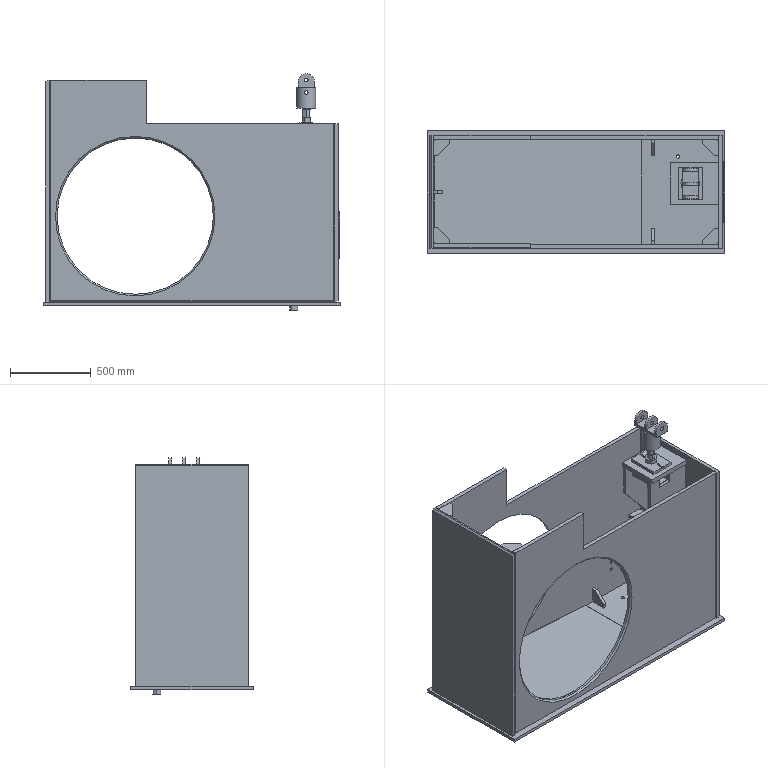Part | SolidWorks | 28 solids | 393 faces | box 1845 x 760 x 1471 mm | volume 146946373 mm3 | plane 246 | cylinder 117 | cone 30 | commonest cylinder face diameters 10.716 x20 14 x20 48 x12 20 x10 22 x6 24 x6